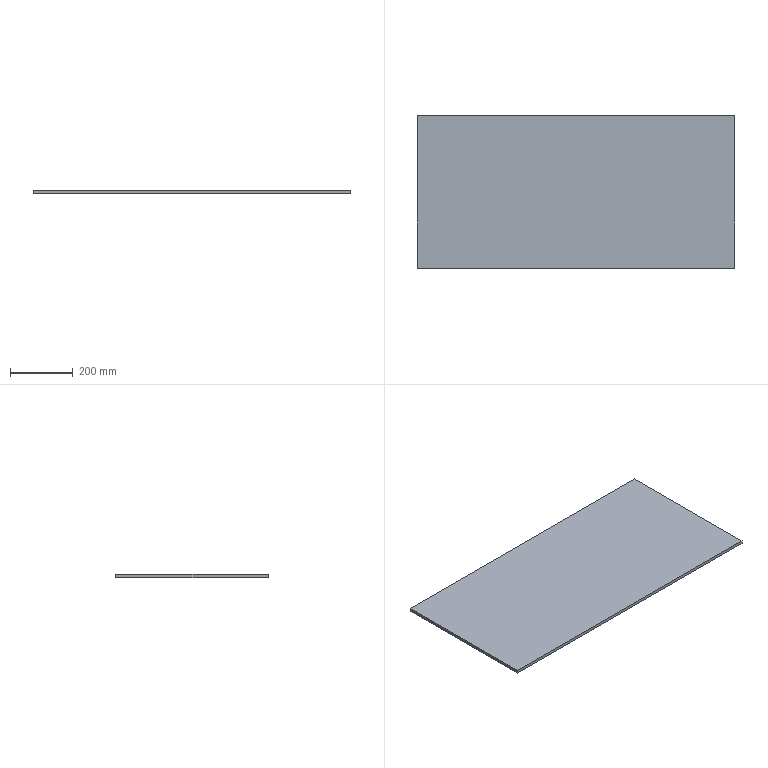Part | NX | features DATUM_CSYS 2, EXTRUDE 1, SKETCH 1 | 1 solid | 6 faces | box 1013 x 485 x 10 mm | volume 4913050 mm3 | plane 6
STEP:
#1=CARTESIAN_POINT('',(0.,0.,0.));
#2=VERTEX_POINT('',#1);
#3=CARTESIAN_POINT('',(1013.,0.,0.));
#4=VERTEX_POINT('',#3);
#5=CARTESIAN_POINT('',(333.,0.,0.));
#6=DIRECTION('',(1.,0.,0.));
#7=VECTOR('',#6,1000.);
#8=LINE('',#5,#7);
#9=EDGE_CURVE('',#2,#4,#8,.T.);
#10=ORIENTED_EDGE('',*,*,#9,.T.);
#11=CARTESIAN_POINT('',(1013.,0.,10.));
#12=VERTEX_POINT('',#11);
#13=CARTESIAN_POINT('',(1013.,0.,10.));
#14=DIRECTION('',(0.,0.,-1.));
#15=VECTOR('',#14,1000.);
#16=LINE('',#13,#15);
#17=EDGE_CURVE('',#12,#4,#16,.T.);
#18=ORIENTED_EDGE('',*,*,#17,.F.);
#19=CARTESIAN_POINT('',(0.,0.,10.));
#20=VERTEX_POINT('',#19);
#21=CARTESIAN_POINT('',(0.,0.,10.));
#22=DIRECTION('',(1.,0.,0.));
#23=VECTOR('',#22,1000.);
#24=LINE('',#21,#23);
#25=EDGE_CURVE('',#20,#12,#24,.T.);
#26=ORIENTED_EDGE('',*,*,#25,.F.);
#27=CARTESIAN_POINT('',(0.,0.,10.));
#28=DIRECTION('',(0.,0.,-1.));
#29=VECTOR('',#28,1000.);
#30=LINE('',#27,#29);
#31=EDGE_CURVE('',#20,#2,#30,.T.);
#32=ORIENTED_EDGE('',*,*,#31,.T.);
#33=EDGE_LOOP('',(#10,#18,#26,#32));
#34=FACE_BOUND('',#33,.T.);
#35=CARTESIAN_POINT('',(333.,0.,10.));
#36=DIRECTION('',(0.,1.,0.));
#37=DIRECTION('',(-1.,0.,0.));
#38=AXIS2_PLACEMENT_3D('',#35,#36,#37);
#39=PLANE('',#38);
#40=ADVANCED_FACE('',(#34),#39,.F.);
#41=CARTESIAN_POINT('',(1013.,485.,0.));
#42=VERTEX_POINT('',#41);
#43=CARTESIAN_POINT('',(1013.,0.,0.));
#44=DIRECTION('',(0.,1.,0.));
#45=VECTOR('',#44,1000.);
#46=LINE('',#43,#45);
#47=EDGE_CURVE('',#4,#42,#46,.T.);
#48=ORIENTED_EDGE('',*,*,#47,.T.);
#49=CARTESIAN_POINT('',(1013.,485.,10.));
#50=VERTEX_POINT('',#49);
#51=CARTESIAN_POINT('',(1013.,485.,10.));
#52=DIRECTION('',(0.,0.,-1.));
#53=VECTOR('',#52,1000.);
#54=LINE('',#51,#53);
#55=EDGE_CURVE('',#50,#42,#54,.T.);
#56=ORIENTED_EDGE('',*,*,#55,.F.);
#57=CARTESIAN_POINT('',(1013.,0.,10.));
#58=DIRECTION('',(0.,1.,0.));
#59=VECTOR('',#58,1000.);
#60=LINE('',#57,#59);
#61=EDGE_CURVE('',#12,#50,#60,.T.);
#62=ORIENTED_EDGE('',*,*,#61,.F.);
#63=ORIENTED_EDGE('',*,*,#17,.T.);
#64=EDGE_LOOP('',(#48,#56,#62,#63));
#65=FACE_BOUND('',#64,.T.);
#66=CARTESIAN_POINT('',(1013.,0.,10.));
#67=DIRECTION('',(-1.,0.,0.));
#68=DIRECTION('',(0.,-1.,0.));
#69=AXIS2_PLACEMENT_3D('',#66,#67,#68);
#70=PLANE('',#69);
#71=ADVANCED_FACE('',(#65),#70,.F.);
#72=CARTESIAN_POINT('',(0.,485.,0.));
#73=VERTEX_POINT('',#72);
#74=CARTESIAN_POINT('',(1013.,485.,0.));
#75=DIRECTION('',(-1.,0.,0.));
#76=VECTOR('',#75,1000.);
#77=LINE('',#74,#76);
#78=EDGE_CURVE('',#42,#73,#77,.T.);
#79=ORIENTED_EDGE('',*,*,#78,.T.);
#80=CARTESIAN_POINT('',(0.,485.,10.));
#81=VERTEX_POINT('',#80);
#82=CARTESIAN_POINT('',(0.,485.,10.));
#83=DIRECTION('',(0.,0.,-1.));
#84=VECTOR('',#83,1000.);
#85=LINE('',#82,#84);
#86=EDGE_CURVE('',#81,#73,#85,.T.);
#87=ORIENTED_EDGE('',*,*,#86,.F.);
#88=CARTESIAN_POINT('',(1013.,485.,10.));
#89=DIRECTION('',(-1.,0.,0.));
#90=VECTOR('',#89,1000.);
#91=LINE('',#88,#90);
#92=EDGE_CURVE('',#50,#81,#91,.T.);
#93=ORIENTED_EDGE('',*,*,#92,.F.);
#94=ORIENTED_EDGE('',*,*,#55,.T.);
#95=EDGE_LOOP('',(#79,#87,#93,#94));
#96=FACE_BOUND('',#95,.T.);
#97=CARTESIAN_POINT('',(1013.,485.,10.));
#98=DIRECTION('',(0.,-1.,0.));
#99=DIRECTION('',(1.,0.,0.));
#100=AXIS2_PLACEMENT_3D('',#97,#98,#99);
#101=PLANE('',#100);
#102=ADVANCED_FACE('',(#96),#101,.F.);
#103=CARTESIAN_POINT('',(0.,485.,0.));
#104=DIRECTION('',(0.,-1.,0.));
#105=VECTOR('',#104,1000.);
#106=LINE('',#103,#105);
#107=EDGE_CURVE('',#73,#2,#106,.T.);
#108=ORIENTED_EDGE('',*,*,#107,.T.);
#109=ORIENTED_EDGE('',*,*,#31,.F.);
#110=CARTESIAN_POINT('',(0.,177.,10.));
#111=DIRECTION('',(0.,-1.,0.));
#112=VECTOR('',#111,1000.);
#113=LINE('',#110,#112);
#114=EDGE_CURVE('',#81,#20,#113,.T.);
#115=ORIENTED_EDGE('',*,*,#114,.F.);
#116=ORIENTED_EDGE('',*,*,#86,.T.);
#117=EDGE_LOOP('',(#108,#109,#115,#116));
#118=FACE_BOUND('',#117,.T.);
#119=CARTESIAN_POINT('',(0.,485.,10.));
#120=DIRECTION('',(1.,0.,0.));
#121=DIRECTION('',(0.,1.,0.));
#122=AXIS2_PLACEMENT_3D('',#119,#120,#121);
#123=PLANE('',#122);
#124=ADVANCED_FACE('',(#118),#123,.F.);
#125=ORIENTED_EDGE('',*,*,#114,.T.);
#126=ORIENTED_EDGE('',*,*,#25,.T.);
#127=ORIENTED_EDGE('',*,*,#61,.T.);
#128=ORIENTED_EDGE('',*,*,#92,.T.);
#129=EDGE_LOOP('',(#125,#126,#127,#128));
#130=FACE_BOUND('',#129,.T.);
#131=CARTESIAN_POINT('',(0.,0.,10.));
#132=DIRECTION('',(0.,0.,1.));
#133=DIRECTION('',(1.,0.,0.));
#134=AXIS2_PLACEMENT_3D('',#131,#132,#133);
#135=PLANE('',#134);
#136=ADVANCED_FACE('',(#130),#135,.T.);
#137=ORIENTED_EDGE('',*,*,#9,.F.);
#138=ORIENTED_EDGE('',*,*,#107,.F.);
#139=ORIENTED_EDGE('',*,*,#78,.F.);
#140=ORIENTED_EDGE('',*,*,#47,.F.);
#141=EDGE_LOOP('',(#137,#138,#139,#140));
#142=FACE_BOUND('',#141,.T.);
#143=CARTESIAN_POINT('',(0.,0.,0.));
#144=DIRECTION('',(0.,0.,1.));
#145=DIRECTION('',(1.,0.,0.));
#146=AXIS2_PLACEMENT_3D('',#143,#144,#145);
#147=PLANE('',#146);
#148=ADVANCED_FACE('',(#142),#147,.F.);
#149=CLOSED_SHELL('',(#40,#71,#102,#124,#136,#148));
#150=MANIFOLD_SOLID_BREP('',#149);
#151=(LENGTH_UNIT()NAMED_UNIT(*)SI_UNIT(.MILLI.,.METRE.));
#152=UNCERTAINTY_MEASURE_WITH_UNIT(LENGTH_MEASURE(0.00001),#151,'','');
#153=(NAMED_UNIT(*)PLANE_ANGLE_UNIT()SI_UNIT($,.RADIAN.));
#154=(NAMED_UNIT(*)SI_UNIT($,.STERADIAN.)SOLID_ANGLE_UNIT());
#155=(GEOMETRIC_REPRESENTATION_CONTEXT(3)GLOBAL_UNCERTAINTY_ASSIGNED_CONTEXT((#152))GLOBAL_UNIT_ASSIGNED_CONTEXT((#151,#153,#154))REPRESENTATION_CONTEXT('',''));
#156=ADVANCED_BREP_SHAPE_REPRESENTATION('',(#150),#155);